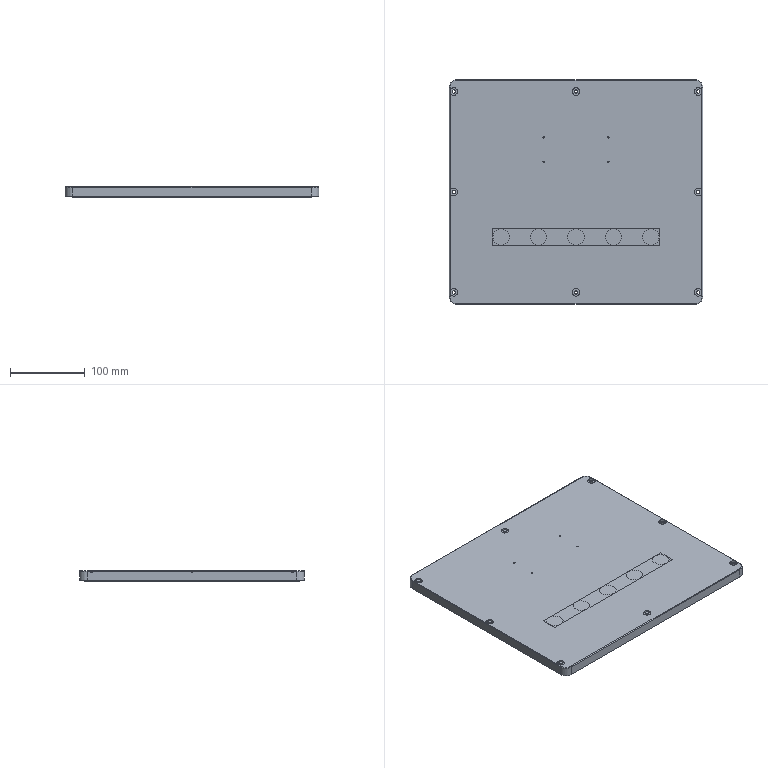NC program | NX | posted with a generic post | part box 338 x 300 x 14.5 mm
Lines 1 to 826 of 9723:
N10 G17 G21 G94 G90
(ADAPTIVE_MILLING_COPY , TOOL : D10)
N12 T04 M6
N14 G54
N16 G17 G0 G90 X-38.397 Y20.082 S9500 M3
N18 G43 Z30. H4
N20 Z1.
N22 G94 G3 X-38.397 Y20.082 Z0.605 I-0.977 J4.393 F1000.
N24 X-38.397 Y20.082 Z0.21 I-0.977 J4.393
N26 X-38.397 Y20.082 Z-0.184 I-0.977 J4.393
N28 X-38.397 Y20.082 Z-0.579 I-0.977 J4.393
N30 X-38.397 Y20.082 Z-0.974 I-0.977 J4.393
N32 X-38.397 Y20.082 Z-1.369 I-0.977 J4.393
N34 X-38.397 Y20.082 Z-1.764 I-0.977 J4.393
N36 X-38.397 Y20.082 Z-2.158 I-0.977 J4.393
N38 X-38.397 Y20.082 Z-2.553 I-0.977 J4.393
N40 X-38.397 Y20.082 Z-2.948 I-0.977 J4.393
N42 X-38.397 Y20.082 Z-3.343 I-0.977 J4.393
N44 X-38.397 Y20.082 Z-3.738 I-0.977 J4.393
N46 X-38.397 Y20.082 Z-4.133 I-0.977 J4.393
N48 X-38.397 Y20.082 Z-4.527 I-0.977 J4.393
N50 X-38.397 Y20.082 Z-4.922 I-0.977 J4.393
N52 X-38.397 Y20.082 Z-5.317 I-0.977 J4.393
N54 X-38.397 Y20.082 Z-5.712 I-0.977 J4.393
N56 X-38.397 Y20.082 Z-6.107 I-0.977 J4.393
N58 X-38.397 Y20.082 Z-6.501 I-0.977 J4.393
N60 X-38.397 Y20.082 Z-6.896 I-0.977 J4.393
N62 X-38.397 Y20.082 Z-7.291 I-0.977 J4.393
N64 X-38.397 Y20.082 Z-7.686 I-0.977 J4.393
N66 X-38.397 Y20.082 Z-8.081 I-0.977 J4.393
N68 X-38.397 Y20.082 Z-8.475 I-0.977 J4.393
N70 X-38.397 Y20.082 Z-8.87 I-0.977 J4.393
N72 X-38.397 Y20.082 Z-9.265 I-0.977 J4.393
N74 X-34.874 Y24.474 Z-9.35 R4.5
N76 X-35.695 Y21.869 R-4.501 F3000.
N78 X-40.367 Y29.338 R4.668
N80 X-35.784 Y21.013 R-4.973
N82 X-41.041 Y29.665 R5.186
N84 X-35.672 Y20.424 R-5.465
N86 X-41.507 Y30.044 R5.705
N88 X-35.522 Y19.864 R-5.982
N90 X-41.742 Y30.524 R6.236
N92 X-35.612 Y19.122 R-6.518
N94 X-41.718 Y31.122 R6.784
N96 X-35.667 Y18.415 R-7.074
N98 X-41.778 Y31.709 R7.356
N100 X-35.662 Y17.749 R-7.651
N102 X-42.325 Y32.139 R7.943
N104 X-35.564 Y17.126 R-8.244
N106 X-42.241 Y32.814 R8.544
N108 X-35.723 Y16.367 R-8.854
N110 X-42.292 Y33.457 R9.165
N112 X-36.17 Y15.51 R-9.482
N114 X-42.079 Y34.188 R9.8
N116 X-36.493 Y14.732 R-10.121
N118 X-42.043 Y34.873 R10.448
N120 X-49.78 Y21.741 R10.778
N122 X-36.636 Y14.007 R10.778
N124 X-28.665 Y27.547 R11.11
N126 X-42.231 Y35.511 R11.11
N128 X-37.491 Y13.145 R11.443
N130 X-27.783 Y26.68 R11.778
N132 X-41.242 Y36.4 R11.778
N134 X-40.107 Y12.34 R12.114
N136 X-39.971 Y37.209 R-12.452
N138 X-43.502 Y12.324 R12.787
N140 X-30.897 Y34.791 R13.109
N142 X-51.814 Y19.209 R13.411
N144 X-26.5 Y19.601 R13.686
N146 X-49.036 Y34.893 R13.965
N148 X-31.673 Y12.368 R14.284
N150 X-43.354 Y38.836 R14.616
N152 X-42.361 Y9.782 R14.949
N154 X-33.211 Y38.763 R15.284
N156 X-51.341 Y14.331 R15.613
N158 X-23.341 Y25.295 R15.908
N160 X-54.062 Y31.793 R16.2
N162 X-28.423 Y12.013 R16.516
N164 X-44.968 Y40.667 R16.847
N166 X-40.14 Y7.254 R17.19
N168 X-31.163 Y40.255 R17.524
N170 X-54.585 Y14.99 R17.838
N172 X-21.715 Y19.908 R18.125
N174 X-54.053 Y36.013 R18.433
N176 X-29.137 Y8.643 R18.775
N178 X-45.862 Y42.777 R19.13
N180 X-39.608 Y4.932 R19.487
N182 X-26.885 Y40.167 R19.819
N184 X-59.148 Y20.208 R20.108
N186 X-20.136 Y17.289 R20.409
N188 X-55.303 Y38.151 R20.747
N190 X-28.761 Y6.128 R21.106
N192 X-47.289 Y44.75 R21.477
N194 X-41. Y2.632 R21.843
N196 X-23.17 Y39.914 R22.164
N198 X-61.954 Y25.073 R22.44
N200 X-17.84 Y16.651 R22.761
N202 X-55.855 Y41.05 R23.122
N204 X-27.388 Y4.144 R23.498
N206 X-51.881 Y45.147 R-23.881
N208 X-38.248 Y0.163 R24.262
N210 X-22.396 Y42.549 R24.59
N212 X-64.365 Y23.837 R24.855
N214 X-14.921 Y17.778 R25.184
N216 X-61.611 Y37.561 R25.563
N218 X-18.509 Y8.776 R25.961
N220 X-60.126 Y41.141 R26.363
N222 X-19.252 Y6.587 R26.772
N224 X-60.882 Y41.502 R-27.18
N226 X-19.908 Y4.706 R27.592
N228 X-60.934 Y42.741 R-28.003
N230 X-19.83 Y3.632 R28.419
N232 X-60.181 Y44.8 R-28.831
N234 X-20.037 Y2.324 R29.248
N236 X-55.312 Y49.789 R29.656
N238 X-25.096 Y-2.148 R30.064
N240 X-39.102 Y55.166 R30.455
N242 X-70.069 Y22.074 R30.701
N244 X-10.03 Y13.968 R30.985
N246 X-69.494 Y34.032 R-31.386
N248 X-14.689 Y4.175 R31.787
N250 X-63.854 Y45.758 R32.198
N252 X-17.347 Y0.19 R32.615
N254 X-46.126 Y57.029 R33.019
N256 X-62.883 Y0.744 R33.341
N258 X-5.802 Y28.286 R33.597
N260 X-72.112 Y34.183 R33.951
N262 X-10.51 Y5.519 R34.345
N264 X-69.489 Y42.271 R-34.757
N266 X-15.062 Y-1.191 R35.172
N268 X-43.201 Y60.044 R35.567
N270 X-74.267 Y16.036 R35.814
N272 X-5.14 Y12.436 R36.097
N274 X-73.625 Y37.666 R36.495
N276 X-11.932 Y-0.471 R36.902
N278 X-43.134 Y61.771 R37.291
N280 X-76.306 Y17.321 R37.532
N282 X-4.676 Y8.98 R37.813
N284 X-73.148 Y42.787 R38.208
N286 X-14.764 Y-5.512 R38.613
N288 X-39.059 Y63.658 R38.991
N290 X-77.909 Y16.504 R39.243
N292 X-2.713 Y9.144 R39.547
N294 X-72.851 Y46.628 R39.936
N296 X-14.101 Y-7.208 R40.34
N298 X-39.944 Y65.393 R40.726
N300 X-80.035 Y18.591 R40.987
N302 X-1.928 Y6.648 R41.282
N304 X-72.686 Y49.858 R41.673
N306 X-13.566 Y-9.006 R42.081
N308 X-39.835 Y67.142 R42.472
N310 X-81.041 Y14.491 R42.755
N312 X0.71 Y8.275 R43.043
N314 X-76.226 Y47.843 R43.431
N316 X-13.024 Y-10.793 R43.836
N318 X-38.86 Y68.891 R44.223
N320 X-83.092 Y15.688 R44.503
N322 X1.137 Y4.93 R44.787
N324 X-75.026 Y52.56 R45.178
N326 X-13.095 Y-13.011 R45.587
N328 X-37.155 Y70.595 R45.978
N330 X-83.755 Y11.041 R46.272
N332 X4.713 Y8.886 R46.568
N334 X-80.034 Y48.353 R46.953
N336 X-15.365 Y-16.553 R47.35
N338 X-33.886 Y72.092 R47.735
N340 X-85.452 Y10.531 R48.041
N342 X7.214 Y10.841 R48.344
N344 X-82.076 Y48.349 R48.727
N346 X-16.494 Y-19.197 R49.117
N348 X-31.144 Y73.487 R49.501
N350 X-88.734 Y17.177 R49.798
N352 X5.756 Y2.284 R50.096
N354 X-81.379 Y52.842 R50.485
N356 X-18.877 Y-22.3 R50.882
N358 X-27.152 Y74.466 R51.267
N360 X-90.874 Y20.34 R51.56
N362 X5.594 Y-1.756 R51.865
N364 X-79.608 Y58.139 R52.256
N366 X-23.479 Y-25.914 R52.654
N368 X-21.114 Y74.473 R53.033
N370 X-92.704 Y27.779 R53.32
N372 X3.965 Y-7.45 R53.633
N374 X-77.355 Y63.191 R54.028
N376 X-26.305 Y-28.553 R54.431
N378 X-18.077 Y75.197 R54.814
N380 X-94.488 Y27.974 R55.11
N382 X5.229 Y-8.755 R55.426
N384 X-77.199 Y65.802 R55.818
N386 X-25.935 Y-30.31 R56.222
N388 X-17.202 Y76.775 R56.608
N390 X-96.351 Y26.806 R56.912
N392 X7.324 Y-8.937 R57.225
N394 X-78.048 Y67.457 R57.615
N396 X-26.218 Y-32.224 R58.018
N398 X-15.732 Y78.096 R58.404
N400 X-97.877 Y30.543 R58.709
N402 X5.748 Y-13.858 R59.015
N404 X-75.932 Y71.56 R59.405
N406 X-28.113 Y-34.459 R59.81
N408 X-12.803 Y78.712 R60.199
N410 X-99.274 Y33.75 R60.502
N412 X7.223 Y-14.91 R60.816
N414 X-76.803 Y73.169 R61.211
N416 X-28.276 Y-36.326 R61.616
N418 X-11.509 Y80.085 R62.004
N420 X-101.056 Y34.055 R62.312
N422 X8.504 Y-16.195 R62.624
N424 X-75.625 Y76.271 R63.016
N426 X-30.928 Y-38.572 R63.421
N428 X-7.037 Y79.705 R63.806
N430 X-101.932 Y39.006 R64.108
N432 X6.585 Y-20.954 R64.426
N434 X-73.224 Y79.996 R64.82
N436 X-37.22 Y-40.902 R65.225
N438 X-2.524 Y78.995 R65.61
N440 X-102.761 Y42.971 R65.914
N442 X5.157 Y-24.819 R66.233
N444 X-70.596 Y83.571 R66.629
N446 X-39.048 Y-42.75 R67.037
N448 X0.028 Y79.428 R67.424
N450 X-104.138 Y44.694 R67.729
N452 X3.601 Y-28.533 R68.046
N454 X-63.555 Y88.716 R68.435
N456 X-45.449 Y-44.288 R68.842
N458 X6.092 Y76.94 R69.229
N460 X-105.173 Y47.352 R69.538
N462 X3.003 Y-31.311 R69.861
N464 X-58.499 Y92.287 R70.252
N466 X-45.765 Y-46.089 R70.661
N468 X7.346 Y78.264 R71.049
N470 X-107.067 Y47.461 R71.364
N472 X4.559 Y-32.421 R71.688
N474 X-61.706 Y93.224 R72.079
N476 X-48.045 Y-47.684 R72.488
N478 X10.942 Y77.461 R72.875
N480 X-107.904 Y50.52 R73.186
N482 X3.618 Y-35.394 R73.511
N484 X-59.676 Y95.754 R73.905
N486 X-49.805 Y-49.296 R74.315
N488 X14.084 Y76.931 R74.701
N490 X-107.901 Y55.288 R75.011
N492 X3.114 Y-37.978 R75.338
N494 X-59.4 Y97.73 R75.735
N496 X-52.124 Y-50.787 R76.145
N498 X16.714 Y76.83 R76.531
N500 X-107.964 Y59.385 R76.84
N502 X-1.046 Y-42.724 R77.165
N504 X-52.581 Y101.114 R77.561
N506 X-57.331 Y-51.594 R77.971
N508 X22.009 Y73.488 R78.356
N510 X-107.652 Y63.802 R78.668
N512 X-3.61 Y-46.179 R78.995
N514 X-43.894 Y103.939 R79.387
N516 X-66.456 Y-50.781 R79.793
N518 X28.571 Y67.405 R80.176
N520 X-106.977 Y68.408 R80.492
N522 X-10.078 Y-51.056 R80.821
N524 X-24.618 Y104.538 R81.211
N526 X-78.984 Y-47.089 R81.609
N528 X35.583 Y58.186 R81.992
N530 X-105.985 Y73.08 R82.318
N532 X-13.397 Y-54.193 R82.655
N534 X-14.097 Y103.784 R83.043
N536 X-95.751 Y-37.256 R83.429
N538 X43.316 Y39.218 R83.798
N540 X-102.199 Y80.663 R84.133
N542 X-21.923 Y-58.378 R84.479
N544 X-3.779 Y101.738 R84.87
N546 X-104.219 Y-31.14 R85.255
N548 X46.111 Y32.112 R85.628
N550 X-103.311 Y82.191 R85.976
N552 X-25.52 Y-60.921 R86.325
N554 X2.679 Y100.523 R86.708
N556 X-113.928 Y-20.847 R87.081
N558 X47.954 Y17.043 R87.446
N560 X-98.94 Y89.206 R87.8
N562 X-32.972 Y-63.642 R88.16
N564 X7.701 Y99.703 R88.548
N566 X-118.403 Y-16.657 R88.924
N568 X49.331 Y12.666 R89.29
N570 X-97.334 Y93.082 R89.645
N572 X-34.922 Y-65.611 R90.005
N574 X12.377 Y98.825 R90.392
N576 X-121.882 Y-13.764 R90.769
N578 X50.575 Y8.629 R91.137
N580 X-99.05 Y94.054 R91.494
N582 X-36.466 Y-67.526 R91.856
N584 X14.446 Y99.631 R92.244
N586 X-125.038 Y-11.175 R92.619
N588 X51.762 Y5.052 R92.985
N590 X-94.789 Y99.797 R93.341
N592 X-40.219 Y-69.417 R93.704
N594 X19.327 Y98.259 R94.092
N596 X-129.249 Y-5.146 R94.464
N598 X51.512 Y-3.265 R94.828
N600 X-91.831 Y104.109 R95.186
N602 X-44.749 Y-71.119 R95.553
N604 X23.607 Y97.108 R95.941
N606 X-133.155 Y1.829 R96.312
N608 X50.314 Y-12.13 R96.675
N610 X-89.318 Y107.876 R97.037
N612 X-55.492 Y-71.772 R97.401
N614 X33.143 Y90.358 R97.782
N616 X-137.611 Y27.832 R98.138
N618 X39.833 Y-34.4 R98.495
N620 X-79.859 Y114.881 R98.87
N622 X-64.014 Y-71.857 R99.248
N624 X39.588 Y85.545 R99.629
N626 X-136.423 Y49.093 R99.973
N628 X27.084 Y-50.939 R100.322
N630 X-70.587 Y120.429 R100.706
N632 X-70.208 Y-72.007 R101.099
N634 X45.853 Y79.911 R101.481
N636 X-132.45 Y66.092 R101.812
N638 X15.801 Y-61.736 R102.156
N640 X-61.853 Y124.74 R102.55
N642 X-75.358 Y-72.193 R102.955
N644 X47.398 Y80.956 R103.344
N646 X-132.06 Y71.235 R103.674
N648 X13.066 Y-65.581 R104.012
N650 X-59.655 Y127.104 R104.408
N652 X-79.379 Y-72.615 R104.814
N654 X49.053 Y81.832 R105.207
N656 X-132.053 Y75.249 R105.541
N658 X8.731 Y-70.056 R105.871
N660 X-55.811 Y129.671 R106.264
N662 X-80.854 Y-74.02 R106.675
N664 X50.769 Y82.612 R107.071
N666 X-133.328 Y76.803 R107.407
N668 X9.399 Y-71.809 R107.737
N670 X-53.277 Y131.916 R108.129
N672 X-83.723 Y-74.808 R108.54
N674 X52.499 Y83.375 R108.938
N676 X-94.486 Y118.891 R109.212
N678 X-148.85 Y27.159 R109.288
N680 X-148.794 Y19.211 R163.374
N682 X-48.966 Y-84.85 R109.677
N684 G1 X-30.591
N686 X-30.366 Y-84.839
N688 G3 X0.806 Y-77.717 R104.864
N690 X-25.916 Y133.85 R109.997
N692 G1 X-51.566
N694 X-51.865 Y133.835
N696 G3 X-67.936 Y130.954 R87.392
N698 X-148.85 Y39.083 R110.28
N700 G1 Y11.034
N702 X-148.834 Y10.735
N704 G3 X-146.474 Y-2.769 R81.81
N706 X-56.67 Y-84.85 R110.559
N708 G1 X-48.945
N710 X-56.67
N712 G2 X-63.51 Y-84.102 R26.56
N714 X-148.745 Y5.315 R110.871
N716 G1 X-148.839 Y5.908
N718 X-148.849 Y5.982
N720 X-148.85 Y5.997
N722 Y11.097
N724 Y5.997
N726 G3 X-148.771 Y1.575 R43.992
N728 X-146.319 Y-8.929 R61.831
N730 X-64.512 Y-84.847 R111.845
N732 G1 X-64.481 Y-84.85
N734 X-58.256
N736 X-64.481
N738 G2 X-69.585 Y-84.12 R17.606
N740 X-108.056 Y-64.913 R109.989
N742 X-148.202 Y-4.32 R112.017
N744 G1 X-148.344 Y-3.737
N746 X-148.414 Y-3.445
N748 X-148.531 Y-2.933
N750 X-148.644 Y-2.42
N752 X-148.722 Y-2.054
N754 X-148.811 Y-1.613
N756 X-148.84 Y-1.465
N758 X-148.85 Y-1.381
N760 Y2.594
N762 Y-1.381
N764 G3 X-147.983 Y-8.419 R20.986
N766 X-137.766 Y-32.364 R105.328
N768 X-71.84 Y-84.485 R113.218
N770 G1 X-71.334 Y-84.626
N772 X-70.9 Y-84.745
N774 X-70.61 Y-84.821
N776 X-70.537 Y-84.837
N778 X-70.462 Y-84.847
N780 X-70.43 Y-84.85
N782 X-65.33
N784 X-70.43
N786 G2 X-74.703 Y-84.139 R13.809
N788 X-98.087 Y-73.569 R105.092
N790 X-147.507 Y-12.006 R113.639
N792 X-148.85 Y-7.125 R55.775
N794 G1 Y-3.675
N796 Y-7.125
N798 G3 X-147.966 Y-13.327 R17.259
N800 X-139.796 Y-31.899 R99.575
N802 X-78.147 Y-84.027 R114.68
N804 X-75.49 Y-84.85 R64.051
N806 G1 X-70.99
N808 X-75.49
N810 G2 X-79.377 Y-84.111 R11.929
N812 X-96.535 Y-76.255 R98.186
N814 X-146.863 Y-18.243 R115.106
N816 X-148.85 Y-12.035 R46.12
N818 G1 Y-8.885
N820 Y-12.035
N822 G3 X-147.924 Y-17.773 R14.897
N824 X-141.578 Y-31.838 R88.751
N826 X-83.704 Y-83.539 R116.148
N828 X-79.957 Y-84.85 R27.189
N830 G1 X-75.907
N832 X-79.957
N834 G2 X-83.466 Y-84.134 R10.264
N836 X-96.951 Y-77.78 R88.142
N838 X-146.491 Y-23.101 R116.502
N840 X-148.85 Y-16.424 R42.51
N842 G1 Y-13.499
N844 Y-16.424
N846 G3 X-147.938 Y-21.707 R13.138
N848 X-141.813 Y-34.554 R82.086
N850 X-88.324 Y-83.211 R117.669
N852 X-84.133 Y-84.842 R43.898
N854 G1 X-84.059 Y-84.85
N856 X-80.309
N858 X-84.059
N860 G2 X-87.336 Y-84.129 R9.34
N862 X-98.508 Y-78.663 R79.349
N864 X-146.135 Y-27.519 R117.886
N866 X-148.85 Y-20.45 R39.882
N868 G1 Y-17.75
N870 Y-20.45
N872 G3 X-148.059 Y-25.075 R11.478
N874 X-142.831 Y-35.859 R69.471
N876 X-92.171 Y-83.082 R118.827
N878 X-87.876 Y-84.848 R27.768
N880 G1 X-87.854 Y-84.85
N882 X-84.329
N884 X-87.854
N886 G2 X-91.115 Y-84.064 R8.805
N888 X-102.201 Y-78.264 R78.466
N890 X-145.487 Y-32.197 R119.272
N892 X-148.826 Y-24.341 R44.082
N894 G1 X-148.84 Y-24.267
N896 X-148.85 Y-24.185
N898 Y-21.635
N900 Y-24.185
N902 G3 X-147.979 Y-28.791 R10.895
N904 X-142.202 Y-39.884 R67.909
N906 X-96.216 Y-82.742 R120.153
N908 X-91.494 Y-84.841 R34.37
N910 G1 X-91.419 Y-84.85
N912 X-88.119
N914 X-91.419
N916 G2 X-94.455 Y-84.092 R8.078
N918 X-104.402 Y-78.704 R69.54
N920 X-145.401 Y-35.543 R120.563
N922 X-148.819 Y-27.887 R41.245
N924 X-148.85 Y-25.217 R42.967
N926 G1 Y-27.692
N928 G3 X-148.021 Y-32.002 R10.007
N930 X-142.968 Y-41.529 R58.904
N932 X-99.669 Y-82.602 R121.11
N934 X-94.924 Y-84.832 R36.311
N936 G1 X-94.85 Y-84.844
N938 X-94.781 Y-84.85
N940 X-91.631
N942 X-94.781
N944 G2 X-97.667 Y-84.112 R7.518
N946 X-106.94 Y-78.9 R63.259
N948 X-145.195 Y-38.948 R121.628
N950 X-148.776 Y-31.368 R39.95
N952 G1 X-148.819 Y-31.224
N954 X-148.834 Y-31.15
N956 X-148.846 Y-31.076
N958 X-148.85 Y-31.027
N960 Y-28.627
N962 Y-31.027
N964 G3 X-147.992 Y-35.253 R9.502
N966 X-143.206 Y-43.989 R56.002
N968 X-103.22 Y-82.32 R122.495
N970 X-98.116 Y-84.837 R31.934
N972 G1 X-98.042 Y-84.847
N974 X-98.009 Y-84.85
N976 X-94.934
N978 X-98.009
N980 G2 X-100.952 Y-84.043 R7.377
N982 X-109.982 Y-78.709 R62.65
N984 X-144.67 Y-42.736 R122.587
N986 X-148.651 Y-34.934 R41.889
N988 G1 X-148.722 Y-34.72
N990 X-148.812 Y-34.434
N992 X-148.83 Y-34.361
N994 X-148.842 Y-34.287
N996 X-148.85 Y-34.213
N998 Y-31.963
N1000 Y-34.213
N1002 G3 X-148.027 Y-38.217 R8.921
N1004 X-143.156 Y-46.818 R51.862
N1006 X-106.265 Y-82.25 R123.255
N1008 X-101.274 Y-84.825 R32.604
N1010 G1 X-101.2 Y-84.839
N1012 X-101.115 Y-84.85
N1014 X-98.19
N1016 X-101.115
N1018 G2 X-103.909 Y-84.064 R6.936
N1020 X-111.99 Y-79.187 R56.14
N1022 X-144.625 Y-45.621 R123.706
N1024 X-148.618 Y-38.078 R40.767
N1026 G1 X-148.668 Y-37.937
N1028 X-148.739 Y-37.724
N1030 X-148.808 Y-37.509
N1032 X-148.826 Y-37.437
N1034 X-148.84 Y-37.363
N1036 X-148.85 Y-37.283
N1038 Y-35.108
N1040 Y-37.283
N1042 G3 X-148.037 Y-41.137 R8.507
N1044 X-143.131 Y-49.544 R49.047
N1046 X-109.744 Y-81.838 R124.195
N1048 X-104.29 Y-84.816 R33.063
N1050 X-101.301 Y-84.85 R35.685
N1052 G1 X-104.076
N1054 G2 X-106.726 Y-84.105 R6.398
N1056 X-114.553 Y-79.246 R52.497
N1058 X-144.428 Y-48.651 R124.706
N1060 X-148.502 Y-41.322 R41.218
N1062 X-148.85 Y-40.221 R13.666
N1064 G1 Y-38.046
N1066 Y-40.221
N1068 G3 X-147.976 Y-44.135 R8.33
N1070 X-143.441 Y-51.718 R45.698
N1072 X-112.538 Y-81.805 R124.672
N1074 X-106.837 Y-84.952 R30.52
N1076 G1 X-106.764 Y-84.969
N1078 X-106.69 Y-84.981
N1080 X-106.616 Y-84.988
N1082 X-106.539 Y-84.99
N1084 G2 X-104.301 Y-84.85 R21.328
N1086 G1 X-104.976
N1088 X-105.024 Y-84.852
N1090 X-106.539 Y-84.99
N1092 G2 X-108.989 Y-84.385 R5.243
N1094 X-115.583 Y-80.382 R40.749
N1096 X-144.313 Y-51.462 R124.482
N1098 X-148.437 Y-44.334 R40.207
N1100 X-148.85 Y-43.08 R9.527
N1102 G1 Y-40.98
N1104 Y-43.08
N1106 G3 X-148.001 Y-46.847 R8.003
N1108 X-143.468 Y-54.255 R43.203
N1110 X-115.236 Y-81.783 R124.091
N1112 X-109.448 Y-85.08 R30.922
N1114 X-108.105 Y-85.372 R2.669
N1116 G2 X-106.635 Y-84.999 R18.923
N1118 G1 X-106.784 Y-85.012
N1120 X-106.879 Y-85.03
N1122 X-108.105 Y-85.372
N1124 G2 X-109.944 Y-85.197 R3.2
N1126 X-115.243 Y-82.422 R22.631
N1128 X-131.695 Y-68.708 R112.433
N1130 X-145.538 Y-52.269 R110.344
N1132 X-148.797 Y-46.124 R27.399
N1134 G1 X-148.818 Y-46.052
N1136 X-148.834 Y-45.979
N1138 X-148.846 Y-45.905
N1140 X-148.85 Y-45.852
N1142 Y-43.827
N1144 Y-45.852
N1146 G3 X-147.941 Y-49.678 R7.86
N1148 X-143.151 Y-57.19 R44.112
N1150 X-117.549 Y-81.998 R123.724
N1152 X-111.591 Y-85.449 R31.371
N1154 X-109.64 Y-85.945 R5.74
N1156 X-108.558 Y-85.499 R4.992
N1158 G1 X-108.197 Y-85.398
N1160 X-108.558 Y-85.499
N1162 X-108.648 Y-85.533
N1164 X-109.349 Y-85.875
N1166 G2 X-111.038 Y-85.926 R2.485
N1168 X-115.866 Y-83.736 R16.583
N1170 X-127.049 Y-75.174 R86.446
N1172 X-144.316 Y-56.575 R122.092
N1174 X-148.49 Y-49.653 R35.791
N1176 X-148.85 Y-48.566 R9.087
N1178 G1 Y-46.541
N1180 Y-48.566
N1182 G3 X-147.937 Y-52.314 R7.677
N1184 X-143.383 Y-59.354 R41.498
N1186 X-119.398 Y-82.518 R121.603
N1188 X-113.164 Y-86.084 R29.649
N1190 X-110.834 Y-86.591 R6.458
N1192 X-110.215 Y-86.297 R1.907
N1194 G1 X-109.474 Y-85.936
N1196 X-110.215 Y-86.297
N1198 X-110.297 Y-86.347
N1200 X-110.416 Y-86.434
N1202 G2 X-111.775 Y-86.711 R1.801
N1204 X-116.067 Y-85.215 R11.734
N1206 X-124.488 Y-79.353 R56.982
N1208 X-144.353 Y-59.008 R121.675
N1210 X-148.473 Y-52.317 R34.331
N1212 X-148.85 Y-51.182 R6.943
N1214 G1 Y-49.232
N1216 Y-51.182
N1218 G3 X-148.013 Y-54.72 R7.252
N1220 X-143.375 Y-61.792 R38.457
N1222 X-121.555 Y-82.804 R119.242
N1224 X-114.902 Y-86.691 R31.249
N1226 X-111.764 Y-87.304 R7.335
N1228 G1 X-111.691 Y-87.286
N1230 X-111.62 Y-87.264
N1232 X-111.55 Y-87.237
N1234 X-111.482 Y-87.205
N1236 X-111.416 Y-87.169
N1238 X-111.394 Y-87.156
N1240 X-110.489 Y-86.488
N1242 X-111.394 Y-87.156
N1244 G2 X-112.973 Y-87.484 R2.237
N1246 X-117.499 Y-85.984 R12.116
N1248 X-126.109 Y-80.005 R53.94
N1250 X-144.508 Y-61.252 R118.286
N1252 X-148.494 Y-54.832 R32.173
N1254 X-148.85 Y-53.769 R7.608
N1256 G1 Y-51.819
N1258 Y-53.769
N1260 G3 X-148.019 Y-57.231 R7.034
N1262 X-143.546 Y-63.963 R36.429
N1264 X-122.935 Y-83.648 R115.403
N1266 X-116.319 Y-87.448 R30.69
N1268 X-112.585 Y-88.064 R7.674
N1270 X-111.701 Y-87.382 R2.106
N1272 G1 X-111.459 Y-87.204
N1274 X-111.701 Y-87.382
N1276 X-111.773 Y-87.446
N1278 X-112.114 Y-87.809
N1280 G2 X-113.477 Y-88.321 R1.815
N1282 X-117.887 Y-87.263 R9.996
N1284 X-125.529 Y-82.406 R40.223
N1286 X-144.573 Y-63.566 R114.254
N1288 X-148.487 Y-57.367 R30.59
N1290 X-148.85 Y-56.303 R8.141
N1292 G1 Y-54.428
N1294 Y-56.303
N1296 G3 X-148.029 Y-59.691 R6.821
N1298 X-143.541 Y-66.322 R35.189
N1300 X-124.649 Y-84.242 R110.736
N1302 X-117.575 Y-88.29 R30.945
N1304 X-113.465 Y-88.91 R8.438
N1306 X-112.878 Y-88.623 R1.462
N1308 G1 X-112.211 Y-87.913
N1310 X-112.878 Y-88.623
N1312 G2 X-114.429 Y-89.205 R2.1
N1314 X-119.139 Y-88.129 R10.626
N1316 X-126.931 Y-83.23 R39.283
N1318 X-144.798 Y-65.645 R109.157
N1320 X-148.577 Y-59.629 R27.72
N1322 X-148.85 Y-58.775 R6.899
N1324 G1 Y-56.975
N1326 Y-58.775
N1328 G3 X-148.043 Y-62.088 R6.61
N1330 X-143.598 Y-68.566 R33.663
N1332 X-125.672 Y-85.328 R103.085
N1334 X-118.606 Y-89.234 R29.554
N1336 X-114.264 Y-89.79 R8.767
N1338 X-113.36 Y-89.312 R1.388
N1340 G1 X-113.025 Y-88.792
N1342 X-112.966 Y-88.717
N1344 X-113.025 Y-88.792
N1346 X-113.36 Y-89.312
N1348 G2 X-114.686 Y-90.063 R1.8
N1350 X-119.174 Y-89.488 R8.973
N1352 X-126.183 Y-85.632 R29.759
N1354 X-145.214 Y-67.448 R99.909
N1356 X-148.715 Y-61.703 R23.833
N1358 G1 X-148.767 Y-61.563
N1360 X-148.792 Y-61.492
N1362 X-148.814 Y-61.42
N1364 X-148.831 Y-61.347
N1366 X-148.843 Y-61.273
N1368 X-148.85 Y-61.198
N1370 Y-59.398
N1372 Y-61.198
N1374 G3 X-147.997 Y-64.575 R6.613
N1376 X-143.764 Y-70.656 R32.514
N1378 X-126.663 Y-86.435 R96.766
N1380 X-119.396 Y-90.277 R28.448
N1382 X-114.819 Y-90.69 R8.839
N1384 X-113.927 Y-90.193 R1.45
N1386 G1 X-113.44 Y-89.436
N1388 X-113.927 Y-90.193
N1390 G2 X-115.233 Y-90.99 R1.855
N1392 X-119.741 Y-90.615 R8.857
N1394 X-126.975 Y-86.873 R27.716
N1396 X-145.558 Y-69.314 R92.206
N1398 X-148.801 Y-63.855 R21.033
N1400 X-148.85 Y-61.873 R11.449
N1402 G1 Y-63.598
N1404 G3 X-147.94 Y-67.036 R6.662
N1406 X-143.291 Y-73.461 R33.626
N1408 X-128.032 Y-87.271 R90.511
N1410 X-120.349 Y-91.281 R28.592
N1412 X-115.618 Y-91.693 R9.589
N1414 X-114.315 Y-91.024 R2.047
N1416 G1 X-114.275 Y-90.961
N1418 X-114.239 Y-90.895
N1420 X-114.014 Y-90.344
N1422 X-113.969 Y-90.258
N1424 X-114.014 Y-90.344
N1426 X-114.239 Y-90.895
N1428 G2 X-115.417 Y-91.855 R1.723
N1430 X-119.639 Y-91.904 R7.877
N1432 X-126.929 Y-88.643 R23.518
N1434 X-138.617 Y-79.162 R76.286
N1436 X-146.802 Y-69.906 R65.195
N1438 X-148.845 Y-66.003 R13.995
N1440 G1 X-148.85 Y-65.939
N1442 Y-64.139
N1444 Y-65.939
N1446 G3 X-147.998 Y-69.238 R6.384
N1448 X-143.421 Y-75.529 R31.538
N1450 X-128.451 Y-88.755 R82.671
N1452 X-120.709 Y-92.47 R26.578
N1454 X-115.892 Y-92.626 R9.331
N1456 X-114.643 Y-91.866 R1.999
N1458 G1 X-114.612 Y-91.807
N1460 X-114.272 Y-90.974
N1462 X-114.612 Y-91.807
N1464 G2 X-115.753 Y-92.801 R1.801
N1466 X-120.262 Y-93.004 R8.081
N1468 X-127.684 Y-89.868 R23.103
N1470 X-139.222 Y-80.683 R70.145
N1472 X-146.843 Y-72.127 R59.998
N1474 X-148.838 Y-68.366 R14.485
N1476 G1 X-148.848 Y-68.291
N1478 X-148.85 Y-68.269
N1480 Y-66.469
N1482 Y-68.269
N1484 G3 X-148.01 Y-71.495 R6.218
N1486 X-143.594 Y-77.532 R29.862
N1488 X-129.614 Y-89.733 R76.965
N1490 X-121.51 Y-93.549 R27.04
N1492 X-116.323 Y-93.637 R9.919
N1494 X-114.933 Y-92.805 R2.536
N1496 X-114.693 Y-92.003 R3.912
N1498 G1 X-114.721 Y-92.098
N1500 X-114.81 Y-92.528
N1502 G2 X-115.815 Y-93.662 R1.654
N1504 X-120.139 Y-94.229 R7.538
N1506 X-127.451 Y-91.65 R20.606
N1508 X-138.445 Y-83.484 R59.69
N1510 X-146.692 Y-74.59 R61.002
N1512 X-148.837 Y-70.656 R14.642
N1514 G1 X-148.848 Y-70.582
N1516 X-148.85 Y-70.555
N1518 Y-68.83
N1520 Y-70.555
N1522 G3 X-147.995 Y-73.776 R6.144
N1524 X-143.522 Y-79.769 R29.071
N1526 X-129.73 Y-91.372 R68.995
N1528 X-121.767 Y-94.767 R25.345
N1530 X-116.58 Y-94.64 R9.967
N1532 X-115.097 Y-93.676 R2.826
N1534 X-114.828 Y-92.618 R5.535
N1536 G1 X-114.993 Y-93.427
N1538 G2 X-115.961 Y-94.6 R1.749
N1540 X-120.248 Y-95.399 R7.486
N1542 X-127.656 Y-93.129 R19.639
N1544 X-138.131 Y-85.784 R53.015
N1546 X-146.705 Y-76.789 R58.159
N1548 X-148.834 Y-72.931 R14.593
N1550 G1 X-148.845 Y-72.857
N1552 X-148.85 Y-72.803
N1554 Y-71.153
N1556 Y-72.803
N1558 G3 X-147.986 Y-76.02 R6.082
N1560 X-143.251 Y-82.189 R29.111
N1562 X-129.983 Y-92.893 R62.756
N1564 X-121.76 Y-96.023 R23.981
N1566 X-116.593 Y-95.583 R9.666
N1568 X-115.187 Y-94.514 R2.695
N1570 X-115.02 Y-93.559 R8.504
N1572 G1 X-115.08 Y-93.853
N1574 X-115.091 Y-93.951
N1576 X-115.094 Y-94.152
N1578 G2 X-115.887 Y-95.436 R1.573
N1580 X-120.166 Y-96.568 R7.211
N1582 X-127.742 Y-94.639 R18.851
N1584 X-138.494 Y-87.446 R48.451
N1586 X-146.765 Y-78.89 R53.493
N1588 X-148.844 Y-75.094 R12.832
N1590 G1 X-148.85 Y-75.019
N1592 Y-73.369
N1594 Y-75.019
N1596 G3 X-147.974 Y-78.232 R6.
N1598 X-143.338 Y-84.192 R28.139
N1600 X-130.111 Y-94.452 R57.308
N1602 X-121.701 Y-97.265 R22.794
N1604 X-116.57 Y-96.532 R9.504
N1606 X-115.177 Y-95.327 R2.861
N1608 X-115.096 Y-94.282 R3.893
N1610 G1 X-115.108 Y-95.032
N1612 G2 X-115.868 Y-96.345 R1.692
N1614 X-120.075 Y-97.721 R7.186
N1616 X-127.729 Y-96.153 R18.126
N1618 X-138.197 Y-89.63 R44.181
N1620 X-146.805 Y-80.992 R50.264
N1622 X-148.836 Y-77.337 R13.437
N1624 G1 X-148.847 Y-77.263
N1626 X-148.85 Y-77.222
N1628 Y-75.572
N1630 Y-77.222
N1632 G3 X-147.988 Y-80.363 R5.928
N1634 X-143.46 Y-86.122 R26.544
N1636 X-130.225 Y-95.985 R52.415
N1638 X-121.796 Y-98.481 R22.228
N1640 X-116.488 Y-97.482 R9.634
N1642 X-115.162 Y-96.205 R2.847
N1644 X-115.109 Y-95.154 R5.627
N1646 G1 X-115.118 Y-95.754
N1648 X-115.111 Y-95.837
N1650 X-115.105 Y-95.873